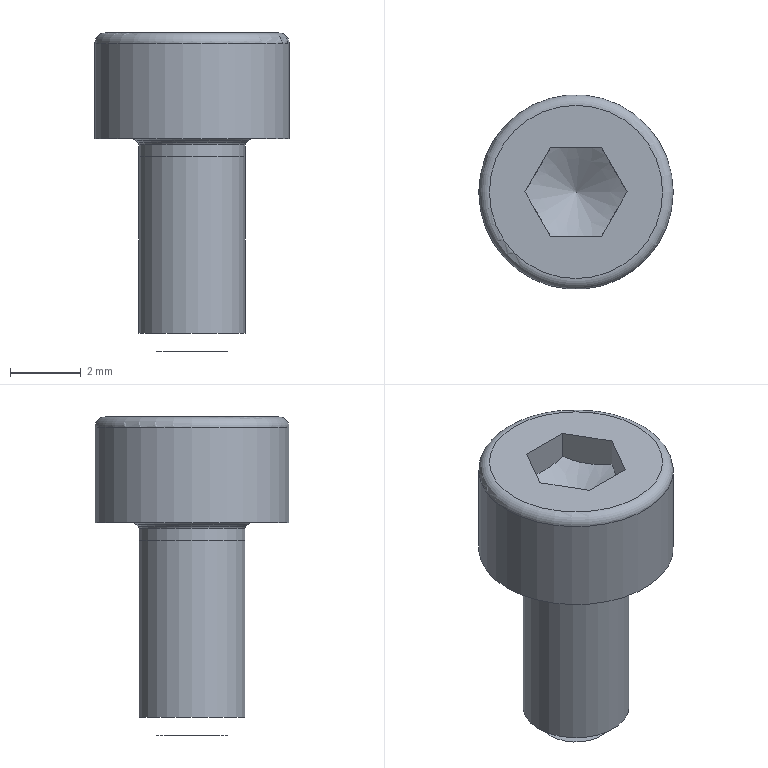Part | NX | features BREP 1, DATUM_CSYS 1 | 1 solid | 18 faces | box 5.5 x 5.5 x 9 mm | volume 106.3 mm3 | plane 9 | cone 3 | torus 3 | cylinder 3 | commonest cylinder face diameters 3 x2 5.5 x1
STEP:
#1=CARTESIAN_POINT('',(-1.443,0.,0.));
#2=VERTEX_POINT('',#1);
#3=CARTESIAN_POINT('',(-1.443,0.,-0.8));
#4=VERTEX_POINT('',#3);
#5=CARTESIAN_POINT('',(-1.443,0.,0.));
#6=DIRECTION('',(0.,0.,-1.));
#7=VECTOR('',#6,1000.);
#8=LINE('',#5,#7);
#9=EDGE_CURVE('',#2,#4,#8,.T.);
#10=ORIENTED_EDGE('',*,*,#9,.T.);
#11=CARTESIAN_POINT('',(-0.7217,1.25,-0.8));
#12=VERTEX_POINT('',#11);
#13=CARTESIAN_POINT('',(-1.443,0.,-0.8));
#14=CARTESIAN_POINT('',(-1.083,0.625,-1.008));
#15=CARTESIAN_POINT('',(-0.7217,1.25,-0.8));
#16=(BOUNDED_CURVE()B_SPLINE_CURVE(2,(#13,#14,#15),.UNSPECIFIED.,.F.,.F.)B_SPLINE_CURVE_WITH_KNOTS((3,3),(0.,1.),.PIECEWISE_BEZIER_KNOTS.)CURVE()GEOMETRIC_REPRESENTATION_ITEM()RATIONAL_B_SPLINE_CURVE((1.,1.155,1.))REPRESENTATION_ITEM(''));
#17=EDGE_CURVE('',#4,#12,#16,.T.);
#18=ORIENTED_EDGE('',*,*,#17,.T.);
#19=CARTESIAN_POINT('',(-0.7217,1.25,0.));
#20=VERTEX_POINT('',#19);
#21=CARTESIAN_POINT('',(-0.7217,1.25,0.));
#22=DIRECTION('',(0.,0.,-1.));
#23=VECTOR('',#22,1000.);
#24=LINE('',#21,#23);
#25=EDGE_CURVE('',#20,#12,#24,.T.);
#26=ORIENTED_EDGE('',*,*,#25,.F.);
#27=CARTESIAN_POINT('',(-1.443,0.,0.));
#28=DIRECTION('',(0.5,0.866,0.));
#29=VECTOR('',#28,1000.);
#30=LINE('',#27,#29);
#31=EDGE_CURVE('',#2,#20,#30,.T.);
#32=ORIENTED_EDGE('',*,*,#31,.F.);
#33=EDGE_LOOP('',(#10,#18,#26,#32));
#34=FACE_BOUND('',#33,.T.);
#35=CARTESIAN_POINT('',(-1.083,0.625,-0.65));
#36=DIRECTION('',(-0.866,0.5,0.));
#37=DIRECTION('',(-0.5,-0.866,0.));
#38=AXIS2_PLACEMENT_3D('',#35,#36,#37);
#39=PLANE('',#38);
#40=ADVANCED_FACE('',(#34),#39,.F.);
#41=ORIENTED_EDGE('',*,*,#25,.T.);
#42=CARTESIAN_POINT('',(0.7217,1.25,-0.8));
#43=VERTEX_POINT('',#42);
#44=CARTESIAN_POINT('',(-0.7217,1.25,-0.8));
#45=CARTESIAN_POINT('',(0.,1.25,-1.008));
#46=CARTESIAN_POINT('',(0.7217,1.25,-0.8));
#47=(BOUNDED_CURVE()B_SPLINE_CURVE(2,(#44,#45,#46),.UNSPECIFIED.,.F.,.F.)B_SPLINE_CURVE_WITH_KNOTS((3,3),(0.,1.),.PIECEWISE_BEZIER_KNOTS.)CURVE()GEOMETRIC_REPRESENTATION_ITEM()RATIONAL_B_SPLINE_CURVE((1.,1.155,1.))REPRESENTATION_ITEM(''));
#48=EDGE_CURVE('',#12,#43,#47,.T.);
#49=ORIENTED_EDGE('',*,*,#48,.T.);
#50=CARTESIAN_POINT('',(0.7217,1.25,0.));
#51=VERTEX_POINT('',#50);
#52=CARTESIAN_POINT('',(0.7217,1.25,0.));
#53=DIRECTION('',(0.,0.,-1.));
#54=VECTOR('',#53,1000.);
#55=LINE('',#52,#54);
#56=EDGE_CURVE('',#51,#43,#55,.T.);
#57=ORIENTED_EDGE('',*,*,#56,.F.);
#58=CARTESIAN_POINT('',(-0.7217,1.25,0.));
#59=DIRECTION('',(1.,0.,0.));
#60=VECTOR('',#59,1000.);
#61=LINE('',#58,#60);
#62=EDGE_CURVE('',#20,#51,#61,.T.);
#63=ORIENTED_EDGE('',*,*,#62,.F.);
#64=EDGE_LOOP('',(#41,#49,#57,#63));
#65=FACE_BOUND('',#64,.T.);
#66=CARTESIAN_POINT('',(0.,1.25,-0.65));
#67=DIRECTION('',(0.,1.,0.));
#68=DIRECTION('',(-1.,0.,0.));
#69=AXIS2_PLACEMENT_3D('',#66,#67,#68);
#70=PLANE('',#69);
#71=ADVANCED_FACE('',(#65),#70,.F.);
#72=ORIENTED_EDGE('',*,*,#56,.T.);
#73=CARTESIAN_POINT('',(1.443,0.,-0.8));
#74=VERTEX_POINT('',#73);
#75=CARTESIAN_POINT('',(0.7217,1.25,-0.8));
#76=CARTESIAN_POINT('',(1.083,0.625,-1.008));
#77=CARTESIAN_POINT('',(1.443,0.,-0.8));
#78=(BOUNDED_CURVE()B_SPLINE_CURVE(2,(#75,#76,#77),.UNSPECIFIED.,.F.,.F.)B_SPLINE_CURVE_WITH_KNOTS((3,3),(0.,1.),.PIECEWISE_BEZIER_KNOTS.)CURVE()GEOMETRIC_REPRESENTATION_ITEM()RATIONAL_B_SPLINE_CURVE((1.,1.155,1.))REPRESENTATION_ITEM(''));
#79=EDGE_CURVE('',#43,#74,#78,.T.);
#80=ORIENTED_EDGE('',*,*,#79,.T.);
#81=CARTESIAN_POINT('',(1.443,0.,0.));
#82=VERTEX_POINT('',#81);
#83=CARTESIAN_POINT('',(1.443,0.,0.));
#84=DIRECTION('',(0.,0.,-1.));
#85=VECTOR('',#84,1000.);
#86=LINE('',#83,#85);
#87=EDGE_CURVE('',#82,#74,#86,.T.);
#88=ORIENTED_EDGE('',*,*,#87,.F.);
#89=CARTESIAN_POINT('',(0.7217,1.25,0.));
#90=DIRECTION('',(0.5,-0.866,0.));
#91=VECTOR('',#90,1000.);
#92=LINE('',#89,#91);
#93=EDGE_CURVE('',#51,#82,#92,.T.);
#94=ORIENTED_EDGE('',*,*,#93,.F.);
#95=EDGE_LOOP('',(#72,#80,#88,#94));
#96=FACE_BOUND('',#95,.T.);
#97=CARTESIAN_POINT('',(1.083,0.625,-0.65));
#98=DIRECTION('',(0.866,0.5,0.));
#99=DIRECTION('',(-0.5,0.866,0.));
#100=AXIS2_PLACEMENT_3D('',#97,#98,#99);
#101=PLANE('',#100);
#102=ADVANCED_FACE('',(#96),#101,.F.);
#103=ORIENTED_EDGE('',*,*,#87,.T.);
#104=CARTESIAN_POINT('',(0.7217,-1.25,-0.8));
#105=VERTEX_POINT('',#104);
#106=CARTESIAN_POINT('',(1.443,0.,-0.8));
#107=CARTESIAN_POINT('',(1.083,-0.625,-1.008));
#108=CARTESIAN_POINT('',(0.7217,-1.25,-0.8));
#109=(BOUNDED_CURVE()B_SPLINE_CURVE(2,(#106,#107,#108),.UNSPECIFIED.,.F.,.F.)B_SPLINE_CURVE_WITH_KNOTS((3,3),(0.,1.),.PIECEWISE_BEZIER_KNOTS.)CURVE()GEOMETRIC_REPRESENTATION_ITEM()RATIONAL_B_SPLINE_CURVE((1.,1.155,1.))REPRESENTATION_ITEM(''));
#110=EDGE_CURVE('',#74,#105,#109,.T.);
#111=ORIENTED_EDGE('',*,*,#110,.T.);
#112=CARTESIAN_POINT('',(0.7217,-1.25,0.));
#113=VERTEX_POINT('',#112);
#114=CARTESIAN_POINT('',(0.7217,-1.25,0.));
#115=DIRECTION('',(0.,0.,-1.));
#116=VECTOR('',#115,1000.);
#117=LINE('',#114,#116);
#118=EDGE_CURVE('',#113,#105,#117,.T.);
#119=ORIENTED_EDGE('',*,*,#118,.F.);
#120=CARTESIAN_POINT('',(1.443,0.,0.));
#121=DIRECTION('',(-0.5,-0.866,0.));
#122=VECTOR('',#121,1000.);
#123=LINE('',#120,#122);
#124=EDGE_CURVE('',#82,#113,#123,.T.);
#125=ORIENTED_EDGE('',*,*,#124,.F.);
#126=EDGE_LOOP('',(#103,#111,#119,#125));
#127=FACE_BOUND('',#126,.T.);
#128=CARTESIAN_POINT('',(1.083,-0.625,-0.65));
#129=DIRECTION('',(0.866,-0.5,0.));
#130=DIRECTION('',(0.5,0.866,0.));
#131=AXIS2_PLACEMENT_3D('',#128,#129,#130);
#132=PLANE('',#131);
#133=ADVANCED_FACE('',(#127),#132,.F.);
#134=ORIENTED_EDGE('',*,*,#118,.T.);
#135=CARTESIAN_POINT('',(-0.7217,-1.25,-0.8));
#136=VERTEX_POINT('',#135);
#137=CARTESIAN_POINT('',(0.7217,-1.25,-0.8));
#138=CARTESIAN_POINT('',(0.,-1.25,-1.008));
#139=CARTESIAN_POINT('',(-0.7217,-1.25,-0.8));
#140=(BOUNDED_CURVE()B_SPLINE_CURVE(2,(#137,#138,#139),.UNSPECIFIED.,.F.,.F.)B_SPLINE_CURVE_WITH_KNOTS((3,3),(0.,1.),.PIECEWISE_BEZIER_KNOTS.)CURVE()GEOMETRIC_REPRESENTATION_ITEM()RATIONAL_B_SPLINE_CURVE((1.,1.155,1.))REPRESENTATION_ITEM(''));
#141=EDGE_CURVE('',#105,#136,#140,.T.);
#142=ORIENTED_EDGE('',*,*,#141,.T.);
#143=CARTESIAN_POINT('',(-0.7217,-1.25,0.));
#144=VERTEX_POINT('',#143);
#145=CARTESIAN_POINT('',(-0.7217,-1.25,0.));
#146=DIRECTION('',(0.,0.,-1.));
#147=VECTOR('',#146,1000.);
#148=LINE('',#145,#147);
#149=EDGE_CURVE('',#144,#136,#148,.T.);
#150=ORIENTED_EDGE('',*,*,#149,.F.);
#151=CARTESIAN_POINT('',(0.7217,-1.25,0.));
#152=DIRECTION('',(-1.,0.,0.));
#153=VECTOR('',#152,1000.);
#154=LINE('',#151,#153);
#155=EDGE_CURVE('',#113,#144,#154,.T.);
#156=ORIENTED_EDGE('',*,*,#155,.F.);
#157=EDGE_LOOP('',(#134,#142,#150,#156));
#158=FACE_BOUND('',#157,.T.);
#159=CARTESIAN_POINT('',(0.,-1.25,-0.65));
#160=DIRECTION('',(0.,-1.,0.));
#161=DIRECTION('',(1.,0.,0.));
#162=AXIS2_PLACEMENT_3D('',#159,#160,#161);
#163=PLANE('',#162);
#164=ADVANCED_FACE('',(#158),#163,.F.);
#165=ORIENTED_EDGE('',*,*,#149,.T.);
#166=CARTESIAN_POINT('',(-0.7217,-1.25,-0.8));
#167=CARTESIAN_POINT('',(-1.083,-0.625,-1.008));
#168=CARTESIAN_POINT('',(-1.443,0.,-0.8));
#169=(BOUNDED_CURVE()B_SPLINE_CURVE(2,(#166,#167,#168),.UNSPECIFIED.,.F.,.F.)B_SPLINE_CURVE_WITH_KNOTS((3,3),(0.,1.),.PIECEWISE_BEZIER_KNOTS.)CURVE()GEOMETRIC_REPRESENTATION_ITEM()RATIONAL_B_SPLINE_CURVE((1.,1.155,1.))REPRESENTATION_ITEM(''));
#170=EDGE_CURVE('',#136,#4,#169,.T.);
#171=ORIENTED_EDGE('',*,*,#170,.T.);
#172=ORIENTED_EDGE('',*,*,#9,.F.);
#173=CARTESIAN_POINT('',(-0.7217,-1.25,0.));
#174=DIRECTION('',(-0.5,0.866,0.));
#175=VECTOR('',#174,1000.);
#176=LINE('',#173,#175);
#177=EDGE_CURVE('',#144,#2,#176,.T.);
#178=ORIENTED_EDGE('',*,*,#177,.F.);
#179=EDGE_LOOP('',(#165,#171,#172,#178));
#180=FACE_BOUND('',#179,.T.);
#181=CARTESIAN_POINT('',(-1.083,-0.625,-0.65));
#182=DIRECTION('',(-0.866,-0.5,0.));
#183=DIRECTION('',(0.5,-0.866,0.));
#184=AXIS2_PLACEMENT_3D('',#181,#182,#183);
#185=PLANE('',#184);
#186=ADVANCED_FACE('',(#180),#185,.F.);
#187=ORIENTED_EDGE('',*,*,#79,.F.);
#188=ORIENTED_EDGE('',*,*,#48,.F.);
#189=ORIENTED_EDGE('',*,*,#17,.F.);
#190=ORIENTED_EDGE('',*,*,#170,.F.);
#191=ORIENTED_EDGE('',*,*,#141,.F.);
#192=ORIENTED_EDGE('',*,*,#110,.F.);
#193=CARTESIAN_POINT('',(0.,0.,-1.633));
#194=VERTEX_POINT('',#193);
#195=CARTESIAN_POINT('',(1.443,0.,-0.8));
#196=DIRECTION('',(-0.866,0.,-0.5));
#197=VECTOR('',#196,1000.);
#198=LINE('',#195,#197);
#199=EDGE_CURVE('',#74,#194,#198,.T.);
#200=ORIENTED_EDGE('',*,*,#199,.T.);
#201=ORIENTED_EDGE('',*,*,#199,.F.);
#202=EDGE_LOOP('',(#187,#188,#189,#190,#191,#192,#200,#201));
#203=FACE_BOUND('',#202,.T.);
#204=CARTESIAN_POINT('',(0.,0.,-1.633));
#205=DIRECTION('',(0.,0.,1.));
#206=DIRECTION('',(-1.,0.,0.));
#207=AXIS2_PLACEMENT_3D('',#204,#205,#206);
#208=CONICAL_SURFACE('',#207,0.,1.047);
#209=ADVANCED_FACE('',(#203),#208,.F.);
#210=CARTESIAN_POINT('',(2.45,0.,0.));
#211=VERTEX_POINT('',#210);
#212=CARTESIAN_POINT('',(0.,0.,0.));
#213=DIRECTION('',(0.,0.,-1.));
#214=DIRECTION('',(1.,0.,0.));
#215=AXIS2_PLACEMENT_3D('',#212,#213,#214);
#216=CIRCLE('',#215,2.45);
#217=EDGE_CURVE('',#211,#211,#216,.T.);
#218=ORIENTED_EDGE('',*,*,#217,.F.);
#219=EDGE_LOOP('',(#218));
#220=FACE_BOUND('',#219,.T.);
#221=ORIENTED_EDGE('',*,*,#124,.T.);
#222=ORIENTED_EDGE('',*,*,#155,.T.);
#223=ORIENTED_EDGE('',*,*,#177,.T.);
#224=ORIENTED_EDGE('',*,*,#31,.T.);
#225=ORIENTED_EDGE('',*,*,#62,.T.);
#226=ORIENTED_EDGE('',*,*,#93,.T.);
#227=EDGE_LOOP('',(#221,#222,#223,#224,#225,#226));
#228=FACE_BOUND('',#227,.T.);
#229=CARTESIAN_POINT('',(0.,0.,0.));
#230=DIRECTION('',(0.,0.,-1.));
#231=DIRECTION('',(-1.,0.,0.));
#232=AXIS2_PLACEMENT_3D('',#229,#230,#231);
#233=PLANE('',#232);
#234=ADVANCED_FACE('',(#220,#228),#233,.F.);
#235=CARTESIAN_POINT('',(2.75,0.,-0.3));
#236=VERTEX_POINT('',#235);
#237=CARTESIAN_POINT('',(2.45,0.,-0.3));
#238=DIRECTION('',(0.,-1.,0.));
#239=DIRECTION('',(1.,0.,0.));
#240=AXIS2_PLACEMENT_3D('',#237,#238,#239);
#241=CIRCLE('',#240,0.3);
#242=EDGE_CURVE('',#236,#211,#241,.T.);
#243=ORIENTED_EDGE('',*,*,#242,.F.);
#244=CARTESIAN_POINT('',(0.,0.,-0.3));
#245=DIRECTION('',(0.,0.,-1.));
#246=DIRECTION('',(1.,0.,0.));
#247=AXIS2_PLACEMENT_3D('',#244,#245,#246);
#248=CIRCLE('',#247,2.75);
#249=EDGE_CURVE('',#236,#236,#248,.T.);
#250=ORIENTED_EDGE('',*,*,#249,.F.);
#251=ORIENTED_EDGE('',*,*,#242,.T.);
#252=ORIENTED_EDGE('',*,*,#217,.T.);
#253=EDGE_LOOP('',(#243,#250,#251,#252));
#254=FACE_BOUND('',#253,.T.);
#255=CARTESIAN_POINT('',(0.,0.,-0.3));
#256=DIRECTION('',(0.,0.,1.));
#257=DIRECTION('',(-1.,0.,0.));
#258=AXIS2_PLACEMENT_3D('',#255,#256,#257);
#259=TOROIDAL_SURFACE('',#258,2.45,0.3);
#260=ADVANCED_FACE('',(#254),#259,.T.);
#261=CARTESIAN_POINT('',(2.75,0.,-3.));
#262=VERTEX_POINT('',#261);
#263=CARTESIAN_POINT('',(0.,0.,-3.));
#264=DIRECTION('',(0.,0.,1.));
#265=DIRECTION('',(1.,0.,0.));
#266=AXIS2_PLACEMENT_3D('',#263,#264,#265);
#267=CIRCLE('',#266,2.75);
#268=EDGE_CURVE('',#262,#262,#267,.T.);
#269=ORIENTED_EDGE('',*,*,#268,.T.);
#270=CARTESIAN_POINT('',(2.75,0.,-3.));
#271=DIRECTION('',(0.,0.,1.));
#272=VECTOR('',#271,1000.);
#273=LINE('',#270,#272);
#274=EDGE_CURVE('',#262,#236,#273,.T.);
#275=ORIENTED_EDGE('',*,*,#274,.T.);
#276=ORIENTED_EDGE('',*,*,#249,.T.);
#277=ORIENTED_EDGE('',*,*,#274,.F.);
#278=EDGE_LOOP('',(#269,#275,#276,#277));
#279=FACE_BOUND('',#278,.T.);
#280=CARTESIAN_POINT('',(0.,0.,-3.));
#281=DIRECTION('',(0.,0.,1.));
#282=DIRECTION('',(-1.,0.,0.));
#283=AXIS2_PLACEMENT_3D('',#280,#281,#282);
#284=CYLINDRICAL_SURFACE('',#283,2.75);
#285=ADVANCED_FACE('',(#279),#284,.T.);
#286=ORIENTED_EDGE('',*,*,#268,.F.);
#287=EDGE_LOOP('',(#286));
#288=FACE_BOUND('',#287,.T.);
#289=CARTESIAN_POINT('',(1.67,0.,-3.));
#290=VERTEX_POINT('',#289);
#291=CARTESIAN_POINT('',(0.,0.,-3.));
#292=DIRECTION('',(0.,0.,1.));
#293=DIRECTION('',(1.,0.,0.));
#294=AXIS2_PLACEMENT_3D('',#291,#292,#293);
#295=CIRCLE('',#294,1.67);
#296=EDGE_CURVE('',#290,#290,#295,.T.);
#297=ORIENTED_EDGE('',*,*,#296,.T.);
#298=EDGE_LOOP('',(#297));
#299=FACE_BOUND('',#298,.T.);
#300=CARTESIAN_POINT('',(0.,0.,-3.));
#301=DIRECTION('',(0.,0.,1.));
#302=DIRECTION('',(-1.,0.,0.));
#303=AXIS2_PLACEMENT_3D('',#300,#301,#302);
#304=PLANE('',#303);
#305=ADVANCED_FACE('',(#288,#299),#304,.F.);
#306=CARTESIAN_POINT('',(1.599,0.,-3.029));
#307=VERTEX_POINT('',#306);
#308=CARTESIAN_POINT('',(0.,0.,-3.029));
#309=DIRECTION('',(0.,0.,1.));
#310=DIRECTION('',(1.,0.,0.));
#311=AXIS2_PLACEMENT_3D('',#308,#309,#310);
#312=CIRCLE('',#311,1.599);
#313=EDGE_CURVE('',#307,#307,#312,.T.);
#314=ORIENTED_EDGE('',*,*,#313,.T.);
#315=CARTESIAN_POINT('',(1.67,0.,-3.1));
#316=DIRECTION('',(0.,1.,0.));
#317=DIRECTION('',(-0.7071,0.,0.7071));
#318=AXIS2_PLACEMENT_3D('',#315,#316,#317);
#319=CIRCLE('',#318,0.1);
#320=EDGE_CURVE('',#307,#290,#319,.T.);
#321=ORIENTED_EDGE('',*,*,#320,.T.);
#322=ORIENTED_EDGE('',*,*,#296,.F.);
#323=ORIENTED_EDGE('',*,*,#320,.F.);
#324=EDGE_LOOP('',(#314,#321,#322,#323));
#325=FACE_BOUND('',#324,.T.);
#326=CARTESIAN_POINT('',(0.,0.,-3.1));
#327=DIRECTION('',(0.,0.,-1.));
#328=DIRECTION('',(-1.,0.,0.));
#329=AXIS2_PLACEMENT_3D('',#326,#327,#328);
#330=TOROIDAL_SURFACE('',#329,1.67,0.1);
#331=ADVANCED_FACE('',(#325),#330,.F.);
#332=CARTESIAN_POINT('',(1.529,0.,-3.099));
#333=VERTEX_POINT('',#332);
#334=CARTESIAN_POINT('',(0.,0.,-3.099));
#335=DIRECTION('',(0.,0.,1.));
#336=DIRECTION('',(1.,0.,0.));
#337=AXIS2_PLACEMENT_3D('',#334,#335,#336);
#338=CIRCLE('',#337,1.529);
#339=EDGE_CURVE('',#333,#333,#338,.T.);
#340=ORIENTED_EDGE('',*,*,#339,.T.);
#341=CARTESIAN_POINT('',(1.529,0.,-3.099));
#342=DIRECTION('',(0.7071,0.,0.7071));
#343=VECTOR('',#342,1000.);
#344=LINE('',#341,#343);
#345=EDGE_CURVE('',#333,#307,#344,.T.);
#346=ORIENTED_EDGE('',*,*,#345,.T.);
#347=ORIENTED_EDGE('',*,*,#313,.F.);
#348=ORIENTED_EDGE('',*,*,#345,.F.);
#349=EDGE_LOOP('',(#340,#346,#347,#348));
#350=FACE_BOUND('',#349,.T.);
#351=CARTESIAN_POINT('',(0.,0.,-3.099));
#352=DIRECTION('',(0.,0.,1.));
#353=DIRECTION('',(-1.,0.,0.));
#354=AXIS2_PLACEMENT_3D('',#351,#352,#353);
#355=CONICAL_SURFACE('',#354,1.529,0.7854);
#356=ADVANCED_FACE('',(#350),#355,.T.);
#357=CARTESIAN_POINT('',(1.5,0.,-3.17));
#358=VERTEX_POINT('',#357);
#359=CARTESIAN_POINT('',(0.,0.,-3.17));
#360=DIRECTION('',(0.,0.,1.));
#361=DIRECTION('',(1.,0.,0.));
#362=AXIS2_PLACEMENT_3D('',#359,#360,#361);
#363=CIRCLE('',#362,1.5);
#364=EDGE_CURVE('',#358,#358,#363,.T.);
#365=ORIENTED_EDGE('',*,*,#364,.T.);
#366=CARTESIAN_POINT('',(1.6,0.,-3.17));
#367=DIRECTION('',(0.,1.,0.));
#368=DIRECTION('',(-1.,0.,0.));
#369=AXIS2_PLACEMENT_3D('',#366,#367,#368);
#370=CIRCLE('',#369,0.1);
#371=EDGE_CURVE('',#358,#333,#370,.T.);
#372=ORIENTED_EDGE('',*,*,#371,.T.);
#373=ORIENTED_EDGE('',*,*,#339,.F.);
#374=ORIENTED_EDGE('',*,*,#371,.F.);
#375=EDGE_LOOP('',(#365,#372,#373,#374));
#376=FACE_BOUND('',#375,.T.);
#377=CARTESIAN_POINT('',(0.,0.,-3.17));
#378=DIRECTION('',(0.,0.,-1.));
#379=DIRECTION('',(-1.,0.,0.));
#380=AXIS2_PLACEMENT_3D('',#377,#378,#379);
#381=TOROIDAL_SURFACE('',#380,1.6,0.1);
#382=ADVANCED_FACE('',(#376),#381,.F.);
#383=CARTESIAN_POINT('',(1.5,0.,-3.5));
#384=VERTEX_POINT('',#383);
#385=CARTESIAN_POINT('',(0.,0.,-3.5));
#386=DIRECTION('',(0.,0.,1.));
#387=DIRECTION('',(1.,0.,0.));
#388=AXIS2_PLACEMENT_3D('',#385,#386,#387);
#389=CIRCLE('',#388,1.5);
#390=EDGE_CURVE('',#384,#384,#389,.T.);
#391=ORIENTED_EDGE('',*,*,#390,.T.);
#392=CARTESIAN_POINT('',(1.5,0.,-3.5));
#393=DIRECTION('',(0.,0.,1.));
#394=VECTOR('',#393,1000.);
#395=LINE('',#392,#394);
#396=EDGE_CURVE('',#384,#358,#395,.T.);
#397=ORIENTED_EDGE('',*,*,#396,.T.);
#398=ORIENTED_EDGE('',*,*,#364,.F.);
#399=ORIENTED_EDGE('',*,*,#396,.F.);
#400=EDGE_LOOP('',(#391,#397,#398,#399));
#401=FACE_BOUND('',#400,.T.);
#402=CARTESIAN_POINT('',(0.,0.,-3.5));
#403=DIRECTION('',(0.,0.,1.));
#404=DIRECTION('',(-1.,0.,0.));
#405=AXIS2_PLACEMENT_3D('',#402,#403,#404);
#406=CYLINDRICAL_SURFACE('',#405,1.5);
#407=ADVANCED_FACE('',(#401),#406,.T.);
#408=ORIENTED_EDGE('',*,*,#390,.F.);
#409=CARTESIAN_POINT('',(1.5,0.,-8.5));
#410=VERTEX_POINT('',#409);
#411=CARTESIAN_POINT('',(1.5,0.,-8.5));
#412=DIRECTION('',(0.,0.,1.));
#413=VECTOR('',#412,1000.);
#414=LINE('',#411,#413);
#415=EDGE_CURVE('',#410,#384,#414,.T.);
#416=ORIENTED_EDGE('',*,*,#415,.F.);
#417=CARTESIAN_POINT('',(0.,0.,-8.5));
#418=DIRECTION('',(0.,0.,-1.));
#419=DIRECTION('',(1.,0.,0.));
#420=AXIS2_PLACEMENT_3D('',#417,#418,#419);
#421=CIRCLE('',#420,1.5);
#422=EDGE_CURVE('',#410,#410,#421,.T.);
#423=ORIENTED_EDGE('',*,*,#422,.F.);
#424=ORIENTED_EDGE('',*,*,#415,.T.);
#425=EDGE_LOOP('',(#408,#416,#423,#424));
#426=FACE_BOUND('',#425,.T.);
#427=CARTESIAN_POINT('',(0.,0.,-9.));
#428=DIRECTION('',(0.,0.,1.));
#429=DIRECTION('',(-1.,0.,0.));
#430=AXIS2_PLACEMENT_3D('',#427,#428,#429);
#431=CYLINDRICAL_SURFACE('',#430,1.5);
#432=ADVANCED_FACE('',(#426),#431,.T.);
#433=CARTESIAN_POINT('',(1.,0.,-9.));
#434=VERTEX_POINT('',#433);
#435=CARTESIAN_POINT('',(0.,0.,-9.));
#436=DIRECTION('',(0.,0.,-1.));
#437=DIRECTION('',(1.,0.,0.));
#438=AXIS2_PLACEMENT_3D('',#435,#436,#437);
#439=CIRCLE('',#438,1.);
#440=EDGE_CURVE('',#434,#434,#439,.T.);
#441=ORIENTED_EDGE('',*,*,#440,.T.);
#442=EDGE_LOOP('',(#441));
#443=FACE_BOUND('',#442,.T.);
#444=CARTESIAN_POINT('',(0.,0.,-9.));
#445=DIRECTION('',(0.,0.,1.));
#446=DIRECTION('',(-1.,0.,0.));
#447=AXIS2_PLACEMENT_3D('',#444,#445,#446);
#448=PLANE('',#447);
#449=ADVANCED_FACE('',(#443),#448,.F.);
#450=ORIENTED_EDGE('',*,*,#440,.F.);
#451=CARTESIAN_POINT('',(1.,0.,-9.));
#452=DIRECTION('',(0.7071,0.,0.7071));
#453=VECTOR('',#452,1000.);
#454=LINE('',#451,#453);
#455=EDGE_CURVE('',#434,#410,#454,.T.);
#456=ORIENTED_EDGE('',*,*,#455,.T.);
#457=ORIENTED_EDGE('',*,*,#422,.T.);
#458=ORIENTED_EDGE('',*,*,#455,.F.);
#459=EDGE_LOOP('',(#450,#456,#457,#458));
#460=FACE_BOUND('',#459,.T.);
#461=CARTESIAN_POINT('',(0.,0.,-9.));
#462=DIRECTION('',(0.,0.,1.));
#463=DIRECTION('',(-1.,0.,0.));
#464=AXIS2_PLACEMENT_3D('',#461,#462,#463);
#465=CONICAL_SURFACE('',#464,1.,0.7854);
#466=ADVANCED_FACE('',(#460),#465,.T.);
#467=CLOSED_SHELL('',(#40,#71,#102,#133,#164,#186,#209,#234,#260,#285,#305,#331,#356,#382,#407,#432,#449,#466));
#468=MANIFOLD_SOLID_BREP('',#467);
#469=(LENGTH_UNIT()NAMED_UNIT(*)SI_UNIT(.MILLI.,.METRE.));
#470=UNCERTAINTY_MEASURE_WITH_UNIT(LENGTH_MEASURE(0.00001),#469,'','');
#471=(NAMED_UNIT(*)PLANE_ANGLE_UNIT()SI_UNIT($,.RADIAN.));
#472=(NAMED_UNIT(*)SI_UNIT($,.STERADIAN.)SOLID_ANGLE_UNIT());
#473=(GEOMETRIC_REPRESENTATION_CONTEXT(3)GLOBAL_UNCERTAINTY_ASSIGNED_CONTEXT((#470))GLOBAL_UNIT_ASSIGNED_CONTEXT((#469,#471,#472))REPRESENTATION_CONTEXT('',''));
#474=ADVANCED_BREP_SHAPE_REPRESENTATION('',(#468),#473);